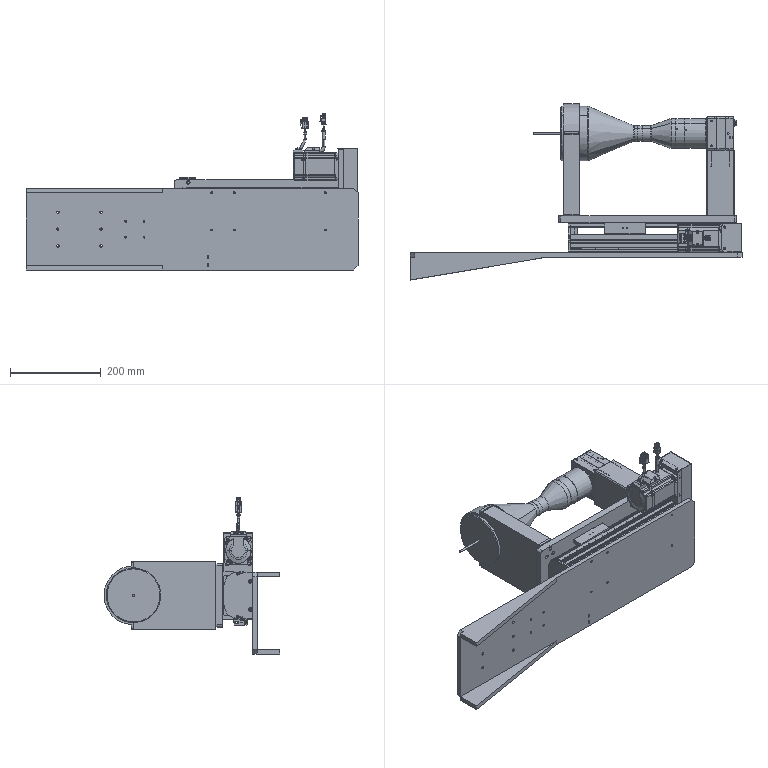Part | SolidWorks | 50 solids | 4059 faces | volume 7028567 mm3 | plane 2329 | cylinder 1405 | cone 249 | spline 68 | torus 8 | commonest cylinder face diameters 2 x116 4.5 x97 3.3 x96 8 x89 4 x67 0.6 x66